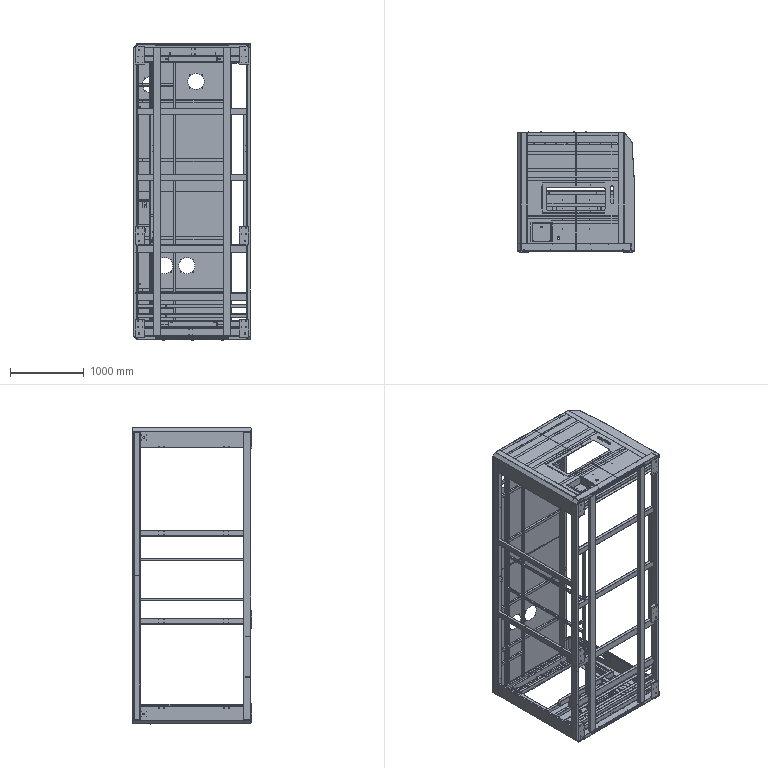Part | SolidWorks | features MirrorCompFeat 1, ReferencePattern 1 | 157 solids | 5415 faces | volume 82035624 mm3 | plane 2831 | cylinder 2338 | cone 184 | spline 46 | torus 16 | commonest cylinder face diameters 3.3 x338 4.2 x296 5 x264 6 x190 0.4 x181 10 x132